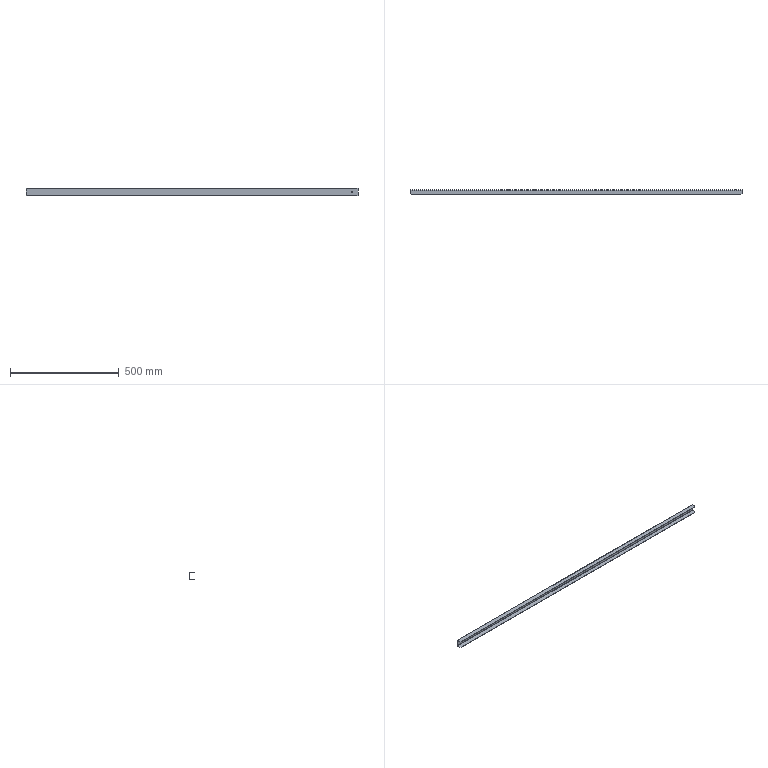Part | STEP file | b-018 | 1 solid | 28 faces | box 1530 x 21.5 x 33 mm | volume 164519 mm3 | plane 22 | cylinder 6 | commonest cylinder face diameters 1.473 x2 3.3 x2 4.473 x2